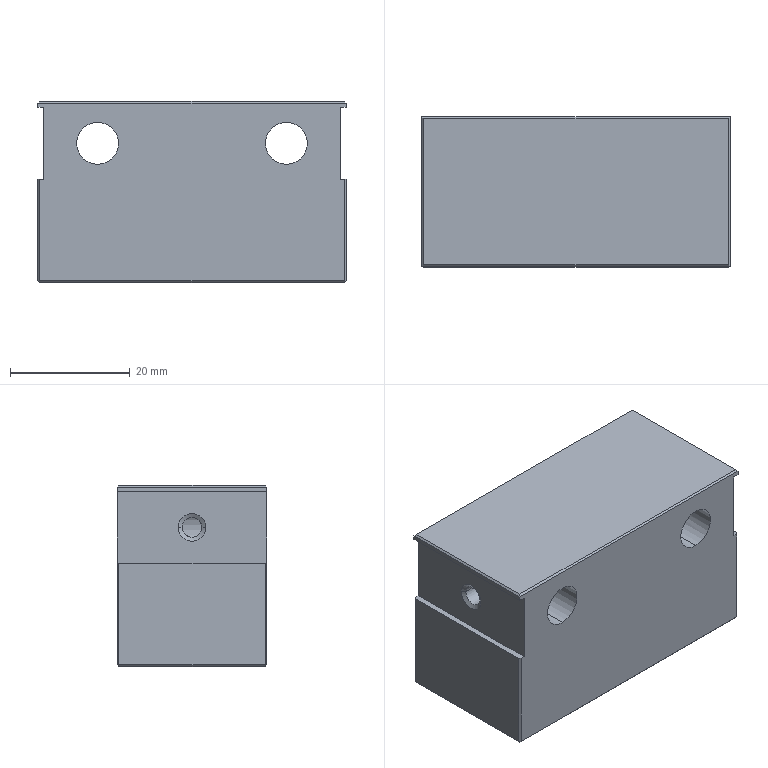Part | NX | 1 solid | 62 faces | box 51.5 x 25 x 30.237 mm | volume 35761 mm3 | plane 26 | cylinder 20 | cone 16 | commonest cylinder face diameters 3.3 x12 4 x4 7 x4